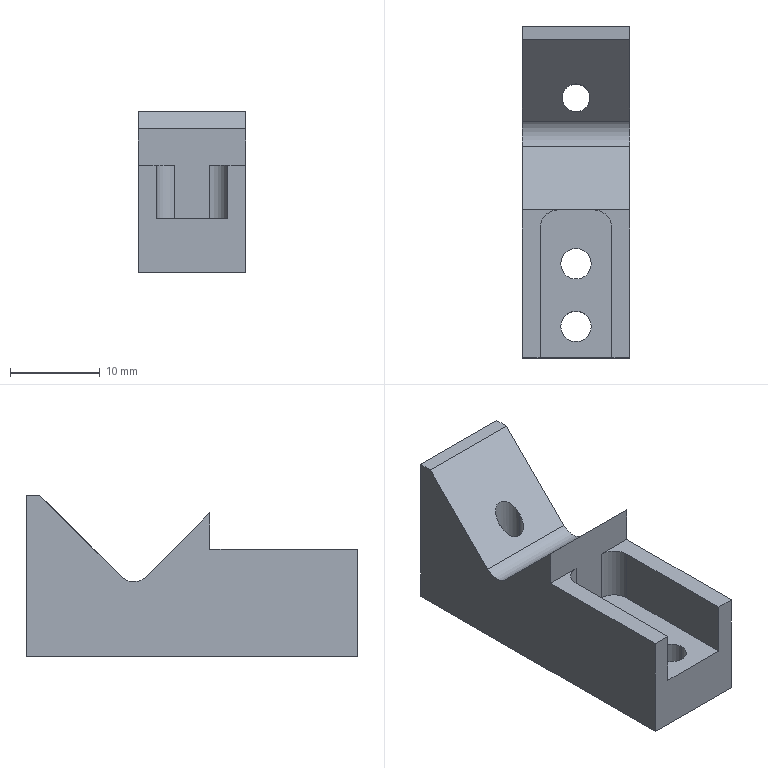Part | STEP file | 1 solid | 31 faces | box 12 x 37 x 18 mm | volume 4359 mm3 | plane 16 | cylinder 15 | commonest cylinder face diameters 3.4 x4 6.5 x4 4 x3 2.5 x2 3.1 x2